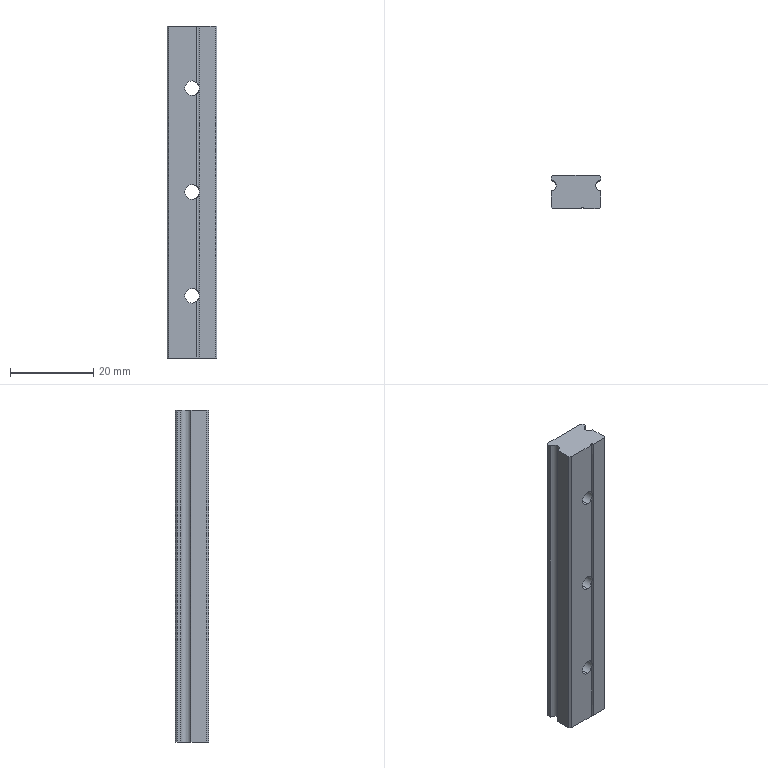Part | STEP file | MGN12H-80-01-CC | 1 solid | 32 faces | box 12 x 8 x 80 mm | volume 6824 mm3 | cylinder 16 | plane 16 | commonest cylinder face diameters 3.5 x6 6 x6 2.5 x3 0.6 x1